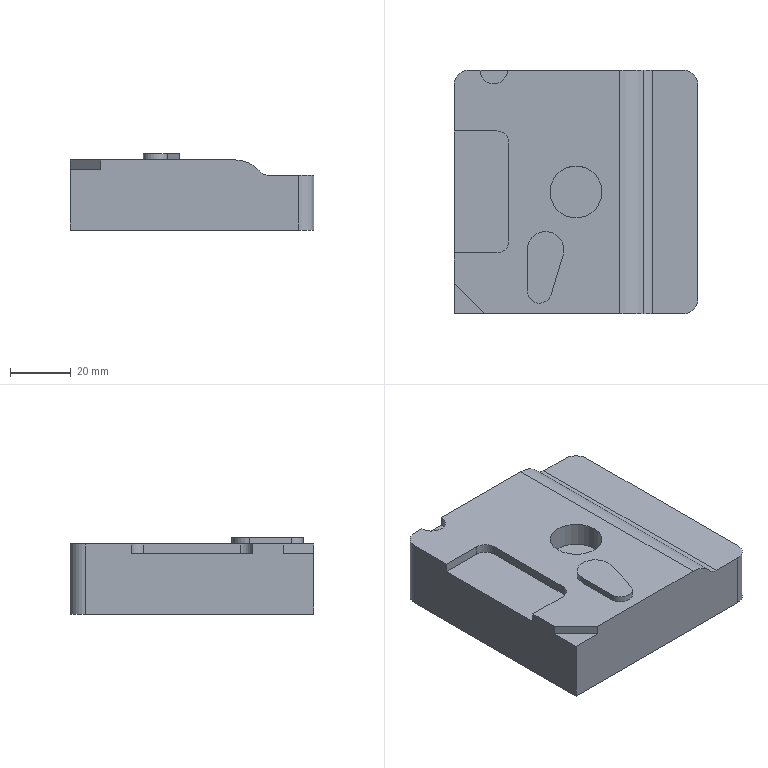NC program | NX | posted with a generic post | part box 80 x 80 x 25 mm
Lines 1 to 1870 of 8300:
N10 G17 G21 G94 G90
(CAVITY_MILL , TOOL : D12D)
N12 T00 M6
N14 G53
N16 G17 G0 G90 X8.231 Y51.991 S0 M3
N18 G43 Z8. H0
N20 Z4.467
N22 G94 G1 Z1.467 F250.
N24 Y41.191
N26 X40.004
N28 G2 X41.191 Y40.004 R1.213
N30 G1 Y-40.004
N32 G2 X40.004 Y-41.191 R1.213
N34 G1 X-4.685
N36 G3 X-1.128 Y-35.794 R11.36
N38 G1 X2.786 Y-22.874
N40 G3 X-23.36 Y-19. R-13.36
N42 G1 Y-32.5
N44 G3 X-19.315 Y-41.191 R11.36
N46 G1 X-18.697 Y-40.457
N48 G2 X-22.4 Y-32.5 R10.4
N50 G1 Y-19.
N52 G2 X1.867 Y-22.595 R-12.4
N54 G1 X-2.047 Y-35.515
N56 G2 X-18.697 Y-40.457 R10.4
N58 G1 X-19.315 Y-41.191
N60 X-40.036
N62 X-40.038
N64 G2 X-40.453 Y-41.11 R1.095
N66 X-41.11 Y-40.453 R1.431
N68 X-41.191 Y-40.038 R1.095
N70 G1 Y-40.036
N72 Y40.004
N74 G2 X-40.004 Y41.191 R1.213
N76 G1 X8.231
N78 Y36.391
N80 X36.391
N82 Y-36.391
N84 X3.706
N86 X7.38 Y-24.265
N88 G3 X-28.16 Y-19. R-18.16
N90 G1 Y-32.5
N92 G3 X-27.684 Y-36.391 R16.16
N94 G1 X-36.391
N96 Y36.391
N98 X8.231
N100 Y31.591
N102 X31.591
N104 Y-31.591
N106 X10.176
N108 X11.974 Y-25.657
N110 G3 X-31.591 Y-11.191 R22.96
N112 G1 Y31.591
N114 X8.231
N116 Y26.791
N118 X26.791
N120 Y-26.791
N122 X16.644
N124 G3 X-26.791 Y3.106 R27.76
N126 G1 Y26.791
N128 X8.231
N130 Y21.991
N132 X21.991
N134 Y-12.942
N136 G3 X-21.991 Y11.271 R32.56
N138 G1 Y21.991
N140 X8.231
N142 Y17.191
N144 X17.191
N146 Y6.62
N148 G3 X-0.729 Y17.191 R37.36
N150 G1 X8.231
N152 Y23.191
N154 Z4.467
N156 G0 Z8.
N158 Y51.992
N160 Z3.933
N162 G1 Z0.933
N164 Y41.192
N166 X40.004
N168 G2 X41.192 Y40.004 R1.213
N170 G1 Y-40.004
N172 G2 X40.004 Y-41.192 R1.213
N174 G1 X-4.685
N176 G3 X-1.128 Y-35.794 R11.36
N178 G1 X2.786 Y-22.874
N180 G3 X-23.36 Y-19. R-13.36
N182 G1 Y-32.5
N184 G3 X-19.315 Y-41.192 R11.36
N186 G1 X-18.697 Y-40.457
N188 G2 X-22.4 Y-32.5 R10.4
N190 G1 Y-19.
N192 G2 X1.867 Y-22.595 R-12.4
N194 G1 X-2.047 Y-35.515
N196 G2 X-18.697 Y-40.457 R10.4
N198 G1 X-19.315 Y-41.192
N200 X-40.036
N202 X-40.037
N204 G2 X-40.453 Y-41.11 R1.097
N206 X-41.11 Y-40.453 R1.43
N208 X-41.192 Y-40.037 R1.097
N210 G1 Y-40.036
N212 Y40.004
N214 G2 X-40.004 Y41.192 R1.213
N216 G1 X8.231
N218 Y36.392
N220 X36.392
N222 Y-36.392
N224 X3.706
N226 X7.38 Y-24.265
N228 G3 X-28.16 Y-19. R-18.16
N230 G1 Y-32.5
N232 G3 X-27.684 Y-36.392 R16.16
N234 G1 X-36.392
N236 Y36.392
N238 X8.231
N240 Y31.592
N242 X31.592
N244 Y-31.592
N246 X10.176
N248 X11.974 Y-25.657
N250 G3 X-31.592 Y-11.192 R22.96
N252 G1 Y31.592
N254 X8.231
N256 Y26.792
N258 X26.792
N260 Y-26.792
N262 X16.644
N264 G3 X-26.792 Y3.106 R27.76
N266 G1 Y26.792
N268 X8.231
N270 Y21.992
N272 X21.992
N274 Y-12.943
N276 G3 X-21.992 Y11.271 R32.56
N278 G1 Y21.992
N280 X8.231
N282 Y17.192
N284 X17.192
N286 Y6.62
N288 G3 X-0.73 Y17.192 R37.36
N290 G1 X8.231
N292 Y23.192
N294 Z3.933
N296 G0 Z8.
N298 Y51.992
N300 Z3.4
N302 G1 Z0.4
N304 Y41.192
N306 X40.004
N308 G2 X41.192 Y40.004 R1.214
N310 G1 Y-40.004
N312 G2 X40.004 Y-41.192 R1.214
N314 G1 X-4.685
N316 G3 X-1.128 Y-35.794 R11.36
N318 G1 X2.786 Y-22.874
N320 G3 X-23.36 Y-19. R-13.36
N322 G1 Y-32.5
N324 G3 X-19.315 Y-41.192 R11.36
N326 G1 X-18.696 Y-40.457
N328 G2 X-22.4 Y-32.5 R10.4
N330 G1 Y-19.
N332 G2 X1.867 Y-22.595 R-12.4
N334 G1 X-2.047 Y-35.515
N336 G2 X-18.696 Y-40.457 R10.4
N338 G1 X-19.315 Y-41.192
N340 X-40.036
N342 X-40.037
N344 G2 X-40.454 Y-41.11 R1.1
N346 X-41.11 Y-40.454 R1.428
N348 X-41.192 Y-40.037 R1.1
N350 G1 Y-40.036
N352 Y40.004
N354 G2 X-40.004 Y41.192 R1.214
N356 G1 X8.231
N358 Y36.392
N360 X36.392
N362 Y-36.392
N364 X3.706
N366 X7.38 Y-24.265
N368 G3 X-28.16 Y-19. R-18.16
N370 G1 Y-32.5
N372 G3 X-27.684 Y-36.392 R16.16
N374 G1 X-36.392
N376 Y36.392
N378 X8.231
N380 Y31.592
N382 X31.592
N384 Y-31.592
N386 X10.176
N388 X11.974 Y-25.657
N390 G3 X-31.592 Y-11.192 R22.96
N392 G1 Y31.592
N394 X8.231
N396 Y26.792
N398 X26.792
N400 Y-26.792
N402 X16.644
N404 G3 X-26.792 Y3.106 R27.76
N406 G1 Y26.792
N408 X8.231
N410 Y21.992
N412 X21.992
N414 Y-12.944
N416 G3 X-21.992 Y11.271 R32.56
N418 G1 Y21.992
N420 X8.231
N422 Y17.192
N424 X17.192
N426 Y6.62
N428 G3 X-0.73 Y17.192 R37.36
N430 G1 X8.231
N432 Y23.192
N434 Z3.4
N436 G0 Z8.
N438 X51.992 Y0.
N440 Z2.8
N442 G1 Z-0.2
N444 X41.192
N446 Y-40.004
N448 G2 X40.004 Y-41.192 R1.214
N450 G1 X23.68
N452 G3 X23.821 Y-39.864 R6.415
N454 G1 Y39.864
N456 G3 X23.68 Y41.192 R6.415
N458 G1 X40.004
N460 G2 X41.192 Y40.004 R1.214
N462 G1 Y0.
N464 X36.392
N466 Y-36.392
N468 X28.621
N470 Y36.392
N472 X36.392
N474 Y0.
N476 X51.992
N478 Z2.8
N480 G0 Z8.
N482 Z2.2
N484 G1 Z-0.8
N486 X41.192
N488 Y-40.003
N490 G2 X40.003 Y-41.192 R1.214
N492 G1 X25.069
N494 G3 X25.19 Y-39.873 R6.258
N496 G1 Y39.873
N498 G3 X25.071 Y41.192 R6.208
N500 G1 X40.003
N502 G2 X41.192 Y40.003 R1.214
N504 G1 Y0.
N506 X36.392
N508 Y-36.392
N510 X29.99
N512 Y36.392
N514 X36.392
N516 Y0.
N518 X51.992
N520 Z2.2
N522 G0 Z8.
N524 Z1.6
N526 G1 Z-1.4
N528 X41.192
N530 Y-40.003
N532 G2 X40.003 Y-41.192 R1.215
N534 G1 X26.043
N536 G3 X26.188 Y-39.731 R6.584
N538 G1 Y39.731
N540 G3 X26.043 Y41.192 R6.584
N542 G1 X40.003
N544 G2 X41.192 Y40.003 R1.215
N546 G1 Y0.
N548 X36.392
N550 Y-36.392
N552 X30.988
N554 Y36.392
N556 X36.392
N558 Y0.
N560 X51.992
N562 Z1.6
N564 G0 Z8.
N566 X51.993 Z1.
N568 G1 Z-2.
N570 X41.193
N572 Y-40.003
N574 G2 X40.003 Y-41.193 R1.215
N576 G1 X26.865
N578 G3 X26.985 Y-39.873 R6.36
N580 G1 Y39.873
N582 G3 X26.865 Y41.193 R6.365
N584 G1 X40.003
N586 G2 X41.193 Y40.003 R1.215
N588 G1 Y0.
N590 X36.393
N592 Y-36.393
N594 X31.785
N596 Y36.393
N598 X36.393
N600 Y0.
N602 X51.993
N604 Z1.
N606 G0 Z8.
N608 Z0.4
N610 G1 Z-2.6
N612 X41.193
N614 Y-40.003
N616 G2 X40.003 Y-41.193 R1.216
N618 G1 X27.517
N620 G3 X27.64 Y-39.874 R6.426
N622 G1 Y39.874
N624 G3 X27.519 Y41.193 R6.397
N626 G1 X40.003
N628 G2 X41.193 Y40.003 R1.216
N630 G1 Y0.
N632 X36.393
N634 Y-36.393
N636 X32.44
N638 Y36.393
N640 X36.393
N642 Y0.
N644 X51.993
N646 Z0.4
N648 G0 Z8.
N650 Z-0.1
N652 G1 Z-3.1
N654 X41.193
N656 Y-40.003
N658 G2 X40.003 Y-41.193 R1.216
N660 G1 X28.009
N662 G3 X28.121 Y-39.873 R6.314
N664 G1 Y39.873
N666 G3 X28.009 Y41.193 R6.314
N668 G1 X40.003
N670 G2 X41.193 Y40.003 R1.216
N672 G1 Y0.
N674 X36.393
N676 Y-36.393
N678 X32.921
N680 Y36.393
N682 X36.393
N684 Y0.
N686 X51.993
N688 Z-0.1
N690 G0 Z8.
N692 Z-0.6
N694 G1 Z-3.6
N696 X41.193
N698 Y-40.003
N700 G2 X40.003 Y-41.193 R1.216
N702 G1 X28.478
N704 G3 X28.574 Y-39.806 R6.174
N706 G1 Y39.806
N708 G3 X28.478 Y41.193 R6.174
N710 G1 X40.003
N712 G2 X41.193 Y40.003 R1.216
N714 G1 Y0.
N716 X36.393
N718 Y-36.393
N720 X33.374
N722 Y36.393
N724 X36.393
N726 Y0.
N728 X51.993
N730 Z-0.6
N732 G0 Z8.
N734 Z-1.1
N736 G1 Z-4.1
N738 X41.193
N740 Y-40.003
N742 G2 X40.003 Y-41.193 R1.217
N744 G1 X29.129
N746 G3 X29.234 Y-39.873 R6.204
N748 G1 Y39.873
N750 G3 X29.129 Y41.193 R6.204
N752 G1 X40.003
N754 G2 X41.193 Y40.003 R1.217
N756 G1 Y0.
N758 X36.393
N760 Y-36.393
N762 X34.034
N764 Y36.393
N766 X36.393
N768 Y0.
N770 X51.993
N772 Z-1.1
N774 G0 Z8.
N776 X51.994 Z-1.6
N778 G1 Z-4.6
N780 X41.194
N782 Y-40.003
N784 G2 X40.003 Y-41.194 R1.217
N786 G1 X30.774
N788 G3 X30.832 Y-39.876 R5.623
N790 G1 Y39.876
N792 G3 X30.781 Y41.194 R5.507
N794 G1 X40.003
N796 G2 X41.194 Y40.003 R1.217
N798 G1 Y0.
N800 X36.394
N802 Y-36.394
N804 X35.632
N806 Y36.394
N808 X36.394
N810 Y0.
N812 X51.994
N814 Z-1.6
N816 G0 Z8.
N818 X32.23 Y52.4
N820 Z-2.2
N822 G1 Z-5.2
N824 Y47.581
N826 X38.016 Y45.994
N828 G2 X45.994 Y38.016 R11.4
N830 G1 X47.581 Y32.23
N832 X52.4
N834 Z-2.2
N836 G0 Z8.
N838 X32.229 Y52.4
N840 Z-2.8
N842 G1 Z-5.8
N844 Y47.581
N846 X38.016 Y45.994
N848 G2 X45.994 Y38.016 R11.4
N850 G1 X47.581 Y32.229
N852 X52.4
N854 Z-2.8
N856 G0 Z8.
N858 X32.228 Y52.4
N860 Z-3.4
N862 G1 Z-6.4
N864 Y47.581
N866 X38.015 Y45.994
N868 G2 X45.994 Y38.015 R11.4
N870 G1 X47.581 Y32.228
N872 X52.4
N874 Z-3.4
N876 G0 Z8.
N878 X32.228 Y52.4
N880 Z-4.
N882 G1 Z-7.
N884 Y47.581
N886 X38.014 Y45.994
N888 G2 X45.994 Y38.014 R11.4
N890 G1 X47.581 Y32.228
N892 X52.4
N894 Z-4.
N896 G0 Z8.
N898 X32.227 Y52.4
N900 Z-4.6
N902 G1 Z-7.6
N904 Y47.58
N906 X38.013 Y45.995
N908 G2 X45.995 Y38.013 R11.4
N910 G1 X47.58 Y32.227
N912 X52.4
N914 Z-4.6
N916 G0 Z8.
N918 X32.226 Y52.4
N920 Z-5.192
N922 G1 Z-8.192
N924 Y47.58
N926 X38.013 Y45.995
N928 G2 X45.995 Y38.013 R11.4
N930 G1 X47.58 Y32.226
N932 X52.4
N934 Z-5.192
N936 G0 Z8.
N938 X32.225 Y52.4
N940 Z-5.785
N942 G1 Z-8.785
N944 Y47.58
N946 X38.012 Y45.995
N948 G2 X45.995 Y38.012 R11.4
N950 G1 X47.58 Y32.225
N952 X52.4
N954 Z-5.785
N956 G0 Z8.
N958 X32.224 Y52.4
N960 Z-6.377
N962 G1 Z-9.377
N964 Y47.58
N966 X38.011 Y45.995
N968 G2 X45.995 Y38.011 R11.4
N970 G1 X47.58 Y32.224
N972 X52.4
N974 Z-6.377
N976 G0 Z8.
N978 X32.223 Y52.4
N980 Z-6.969
N982 G1 Z-9.969
N984 Y47.58
N986 X38.01 Y45.995
N988 G2 X45.995 Y38.01 R11.4
N990 G1 X47.58 Y32.223
N992 X52.4
N994 Z-6.969
N996 G0 Z8.
N998 X32.222 Y52.4
N1000 Z-7.562
N1002 G1 Z-10.562
N1004 Y47.58
N1006 X38.01 Y45.996
N1008 G2 X45.996 Y38.01 R11.4
N1010 G1 X47.58 Y32.222
N1012 X52.4
N1014 Z-7.562
N1016 G0 Z8.
N1018 X32.222 Y52.4
N1020 Z-8.154
N1022 G1 Z-11.154
N1024 Y47.579
N1026 X38.009 Y45.996
N1028 G2 X45.996 Y38.009 R11.4
N1030 G1 X47.579 Y32.222
N1032 X52.4
N1034 Z-8.154
N1036 G0 Z8.
N1038 X32.221 Y52.4
N1040 Z-8.746
N1042 G1 Z-11.746
N1044 Y47.579
N1046 X38.008 Y45.996
N1048 G2 X45.996 Y38.008 R11.4
N1050 G1 X47.579 Y32.221
N1052 X52.4
N1054 Z-8.746
N1056 G0 Z8.
N1058 X32.22 Y52.4
N1060 Z-9.338
N1062 G1 Z-12.338
N1064 Y47.579
N1066 X38.007 Y45.996
N1068 G2 X45.996 Y38.007 R11.4
N1070 G1 X47.579 Y32.22
N1072 X52.4
N1074 Z-9.338
N1076 G0 Z8.
N1078 X32.219 Y52.4
N1080 Z-9.931
N1082 G1 Z-12.931
N1084 Y47.579
N1086 X38.007 Y45.996
N1088 G2 X45.996 Y38.007 R11.4
N1090 G1 X47.579 Y32.219
N1092 X52.4
N1094 Z-9.931
N1096 G0 Z8.
N1098 X32.218 Y52.4
N1100 Z-10.523
N1102 G1 Z-13.523
N1104 Y47.579
N1106 X38.006 Y45.997
N1108 G2 X45.997 Y38.006 R11.4
N1110 G1 X47.579 Y32.218
N1112 X52.4
N1114 Z-10.523
N1116 G0 Z8.
N1118 X32.217 Y52.4
N1120 Z-11.115
N1122 G1 Z-14.115
N1124 Y47.578
N1126 X38.005 Y45.997
N1128 G2 X45.997 Y38.005 R11.4
N1130 G1 X47.578 Y32.217
N1132 X52.4
N1134 Z-11.115
N1136 G0 Z8.
N1138 X32.216 Y52.4
N1140 Z-11.708
N1142 G1 Z-14.708
N1144 Y47.578
N1146 X38.004 Y45.997
N1148 G2 X45.997 Y38.004 R11.4
N1150 G1 X47.578 Y32.216
N1152 X52.4
N1154 Z-11.708
N1156 G0 Z8.
N1158 X32.216 Y52.4
N1160 Z-12.3
N1162 G1 Z-15.3
N1164 Y47.578
N1166 X38.004 Y45.997
N1168 G2 X45.997 Y38.004 R11.4
N1170 G1 X47.578 Y32.216
N1172 X52.4
N1174 Z-12.3
N1176 G0 Z8.
N1178 X32.215 Y52.4
N1180 Z-12.892
N1182 G1 Z-15.892
N1184 Y47.578
N1186 X38.003 Y45.997
N1188 G2 X45.997 Y38.003 R11.4
N1190 G1 X47.578 Y32.215
N1192 X52.4
N1194 Z-12.892
N1196 G0 Z8.
N1198 X32.214 Y52.4
N1200 Z-13.485
N1202 G1 Z-16.485
N1204 Y47.578
N1206 X38.002 Y45.998
N1208 G2 X45.998 Y38.002 R11.4
N1210 G1 X47.578 Y32.214
N1212 X52.4
N1214 Z-13.485
N1216 G0 Z8.
N1218 X32.213 Y52.4
N1220 Z-14.077
N1222 G1 Z-17.077
N1224 Y47.577
N1226 X38.001 Y45.998
N1228 G2 X45.998 Y38.001 R11.4
N1230 G1 X47.577 Y32.213
N1232 X52.4
N1234 Z-14.077
N1236 G0 Z8.
N1238 X32.212 Y52.4
N1240 Z-14.669
N1242 G1 Z-17.669
N1244 Y47.577
N1246 X38.001 Y45.998
N1248 G2 X45.998 Y38.001 R11.4
N1250 G1 X47.577 Y32.212
N1252 X52.4
N1254 Z-14.669
N1256 G0 Z8.
N1258 X32.211 Y52.4
N1260 Z-15.262
N1262 G1 Z-18.262
N1264 Y47.577
N1266 X38. Y45.998
N1268 G2 X45.998 Y38. R11.4
N1270 G1 X47.577 Y32.211
N1272 X52.4
N1274 Z-15.262
N1276 G0 Z8.
N1278 X32.21 Y52.4
N1280 Z-15.854
N1282 G1 Z-18.854
N1284 Y47.577
N1286 X37.999 Y45.998
N1288 G2 X45.998 Y37.999 R11.4
N1290 G1 X47.577 Y32.21
N1292 X52.4
N1294 Z-15.854
N1296 G0 Z8.
N1298 X32.209 Y52.4
N1300 Z-16.446
N1302 G1 Z-19.446
N1304 Y47.577
N1306 X37.998 Y45.999
N1308 G2 X45.999 Y37.998 R11.4
N1310 G1 X47.577 Y32.209
N1312 X52.4
N1314 Z-16.446
N1316 G0 Z8.
N1318 X32.209 Y52.4
N1320 Z-17.038
N1322 G1 Z-20.038
N1324 Y47.576
N1326 X37.997 Y45.999
N1328 G2 X45.999 Y37.997 R11.4
N1330 G1 X47.576 Y32.209
N1332 X52.4
N1334 Z-17.038
N1336 G0 Z8.
N1338 X32.208 Y52.4
N1340 Z-17.631
N1342 G1 Z-20.631
N1344 Y47.576
N1346 X37.997 Y45.999
N1348 G2 X45.999 Y37.997 R11.4
N1350 G1 X47.576 Y32.208
N1352 X52.4
N1354 Z-17.631
N1356 G0 Z8.
N1358 X32.207 Y52.4
N1360 Z-18.223
N1362 G1 Z-21.223
N1364 Y47.576
N1366 X37.996 Y45.999
N1368 G2 X45.999 Y37.996 R11.4
N1370 G1 X47.576 Y32.207
N1372 X52.4
N1374 Z-18.223
N1376 G0 Z8.
N1378 X32.206 Y52.4
N1380 Z-18.815
N1382 G1 Z-21.815
N1384 Y47.576
N1386 X37.995 Y45.999
N1388 G2 X45.999 Y37.995 R11.4
N1390 G1 X47.576 Y32.206
N1392 X52.4
N1394 Z-18.815
N1396 G0 Z8.
N1398 X32.205 Y52.4
N1400 Z-19.408
N1402 G1 Z-22.408
N1404 Y47.576
N1406 X37.994 Y46.
N1408 G2 X46. Y37.994 R11.4
N1410 G1 X47.576 Y32.205
N1412 X52.4
N1414 Z-19.408
N1416 G0 Z8.
N1418 X32.204 Y52.4
N1420 Z-20.
N1422 G1 Z-23.
N1424 Y47.576
N1426 X37.994 Y46.
N1428 G2 X46. Y37.994 R11.4
N1430 G1 X47.576 Y32.204
N1432 X52.4
N1434 Z-20.
N1436 G0 Z8.
N1438 Y-32.23
N1440 Z-2.2
N1442 G1 Z-5.2
N1444 X47.581
N1446 X45.994 Y-38.016
N1448 G2 X38.016 Y-45.994 R11.4
N1450 G1 X32.23 Y-47.581
N1452 Y-52.4
N1454 Z-2.2
N1456 G0 Z8.
N1458 X52.4 Y-32.229
N1460 Z-2.8
N1462 G1 Z-5.8
N1464 X47.581
N1466 X45.994 Y-38.016
N1468 G2 X38.016 Y-45.994 R11.4
N1470 G1 X32.229 Y-47.581
N1472 Y-52.4
N1474 Z-2.8
N1476 G0 Z8.
N1478 X52.4 Y-32.228
N1480 Z-3.4
N1482 G1 Z-6.4
N1484 X47.581
N1486 X45.994 Y-38.015
N1488 G2 X38.015 Y-45.994 R11.4
N1490 G1 X32.228 Y-47.581
N1492 Y-52.4
N1494 Z-3.4
N1496 G0 Z8.
N1498 X52.4 Y-32.228
N1500 Z-4.
N1502 G1 Z-7.
N1504 X47.581
N1506 X45.994 Y-38.014
N1508 G2 X38.014 Y-45.994 R11.4
N1510 G1 X32.228 Y-47.581
N1512 Y-52.4
N1514 Z-4.
N1516 G0 Z8.
N1518 X52.4 Y-32.227
N1520 Z-4.6
N1522 G1 Z-7.6
N1524 X47.58
N1526 X45.995 Y-38.013
N1528 G2 X38.013 Y-45.995 R11.4
N1530 G1 X32.227 Y-47.58
N1532 Y-52.4
N1534 Z-4.6
N1536 G0 Z8.
N1538 X52.4 Y-32.226
N1540 Z-5.192
N1542 G1 Z-8.192
N1544 X47.58
N1546 X45.995 Y-38.013
N1548 G2 X38.013 Y-45.995 R11.4
N1550 G1 X32.226 Y-47.58
N1552 Y-52.4
N1554 Z-5.192
N1556 G0 Z8.
N1558 X52.4 Y-32.225
N1560 Z-5.785
N1562 G1 Z-8.785
N1564 X47.58
N1566 X45.995 Y-38.012
N1568 G2 X38.012 Y-45.995 R11.4
N1570 G1 X32.225 Y-47.58
N1572 Y-52.4
N1574 Z-5.785
N1576 G0 Z8.
N1578 X52.4 Y-32.224
N1580 Z-6.377
N1582 G1 Z-9.377
N1584 X47.58
N1586 X45.995 Y-38.011
N1588 G2 X38.011 Y-45.995 R11.4
N1590 G1 X32.224 Y-47.58
N1592 Y-52.4
N1594 Z-6.377
N1596 G0 Z8.
N1598 X52.4 Y-32.223
N1600 Z-6.969
N1602 G1 Z-9.969
N1604 X47.58
N1606 X45.995 Y-38.01
N1608 G2 X38.01 Y-45.995 R11.4
N1610 G1 X32.223 Y-47.58
N1612 Y-52.4
N1614 Z-6.969
N1616 G0 Z8.
N1618 X52.4 Y-32.222
N1620 Z-7.562
N1622 G1 Z-10.562
N1624 X47.58
N1626 X45.996 Y-38.01
N1628 G2 X38.01 Y-45.996 R11.4
N1630 G1 X32.222 Y-47.58
N1632 Y-52.4
N1634 Z-7.562
N1636 G0 Z8.
N1638 X52.4 Y-32.222
N1640 Z-8.154
N1642 G1 Z-11.154
N1644 X47.579
N1646 X45.996 Y-38.009
N1648 G2 X38.009 Y-45.996 R11.4
N1650 G1 X32.222 Y-47.579
N1652 Y-52.4
N1654 Z-8.154
N1656 G0 Z8.
N1658 X52.4 Y-32.221
N1660 Z-8.746
N1662 G1 Z-11.746
N1664 X47.579
N1666 X45.996 Y-38.008
N1668 G2 X38.008 Y-45.996 R11.4
N1670 G1 X32.221 Y-47.579
N1672 Y-52.4
N1674 Z-8.746
N1676 G0 Z8.
N1678 X52.4 Y-32.22
N1680 Z-9.338
N1682 G1 Z-12.338
N1684 X47.579
N1686 X45.996 Y-38.007
N1688 G2 X38.007 Y-45.996 R11.4
N1690 G1 X32.22 Y-47.579
N1692 Y-52.4
N1694 Z-9.338
N1696 G0 Z8.
N1698 X52.4 Y-32.219
N1700 Z-9.931
N1702 G1 Z-12.931
N1704 X47.579
N1706 X45.996 Y-38.007
N1708 G2 X38.007 Y-45.996 R11.4
N1710 G1 X32.219 Y-47.579
N1712 Y-52.4
N1714 Z-9.931
N1716 G0 Z8.
N1718 X52.4 Y-32.218
N1720 Z-10.523
N1722 G1 Z-13.523
N1724 X47.579
N1726 X45.997 Y-38.006
N1728 G2 X38.006 Y-45.997 R11.4
N1730 G1 X32.218 Y-47.579
N1732 Y-52.4
N1734 Z-10.523
N1736 G0 Z8.
N1738 X52.4 Y-32.217
N1740 Z-11.115
N1742 G1 Z-14.115
N1744 X47.578
N1746 X45.997 Y-38.005
N1748 G2 X38.005 Y-45.997 R11.4
N1750 G1 X32.217 Y-47.578
N1752 Y-52.4
N1754 Z-11.115
N1756 G0 Z8.
N1758 X52.4 Y-32.216
N1760 Z-11.708
N1762 G1 Z-14.708
N1764 X47.578
N1766 X45.997 Y-38.004
N1768 G2 X38.004 Y-45.997 R11.4
N1770 G1 X32.216 Y-47.578
N1772 Y-52.4
N1774 Z-11.708
N1776 G0 Z8.
N1778 X52.4 Y-32.216
N1780 Z-12.3
N1782 G1 Z-15.3
N1784 X47.578
N1786 X45.997 Y-38.004
N1788 G2 X38.004 Y-45.997 R11.4
N1790 G1 X32.216 Y-47.578
N1792 Y-52.4
N1794 Z-12.3
N1796 G0 Z8.
N1798 X52.4 Y-32.215
N1800 Z-12.892
N1802 G1 Z-15.892
N1804 X47.578
N1806 X45.997 Y-38.003
N1808 G2 X38.003 Y-45.997 R11.4
N1810 G1 X32.215 Y-47.578
N1812 Y-52.4
N1814 Z-12.892
N1816 G0 Z8.
N1818 X52.4 Y-32.214
N1820 Z-13.485
N1822 G1 Z-16.485
N1824 X47.578
N1826 X45.998 Y-38.002
N1828 G2 X38.002 Y-45.998 R11.4
N1830 G1 X32.214 Y-47.578
N1832 Y-52.4
N1834 Z-13.485
N1836 G0 Z8.
N1838 X52.4 Y-32.213
N1840 Z-14.077
N1842 G1 Z-17.077
N1844 X47.577
N1846 X45.998 Y-38.001
N1848 G2 X38.001 Y-45.998 R11.4
N1850 G1 X32.213 Y-47.577
N1852 Y-52.4
N1854 Z-14.077
N1856 G0 Z8.
N1858 X52.4 Y-32.212
N1860 Z-14.669
N1862 G1 Z-17.669
N1864 X47.577
N1866 X45.998 Y-38.001
N1868 G2 X38.001 Y-45.998 R11.4
N1870 G1 X32.212 Y-47.577
N1872 Y-52.4
N1874 Z-14.669
N1876 G0 Z8.
N1878 X52.4 Y-32.211
N1880 Z-15.262
N1882 G1 Z-18.262
N1884 X47.577
N1886 X45.998 Y-38.
N1888 G2 X38. Y-45.998 R11.4
N1890 G1 X32.211 Y-47.577
N1892 Y-52.4
N1894 Z-15.262
N1896 G0 Z8.
N1898 X52.4 Y-32.21
N1900 Z-15.854
N1902 G1 Z-18.854
N1904 X47.577
N1906 X45.998 Y-37.999
N1908 G2 X37.999 Y-45.998 R11.4
N1910 G1 X32.21 Y-47.577
N1912 Y-52.4
N1914 Z-15.854
N1916 G0 Z8.
N1918 X52.4 Y-32.209
N1920 Z-16.446
N1922 G1 Z-19.446
N1924 X47.577
N1926 X45.999 Y-37.998
N1928 G2 X37.998 Y-45.999 R11.4
N1930 G1 X32.209 Y-47.577
N1932 Y-52.4
N1934 Z-16.446
N1936 G0 Z8.
N1938 X52.4 Y-32.209
N1940 Z-17.038
N1942 G1 Z-20.038
N1944 X47.576
N1946 X45.999 Y-37.997
N1948 G2 X37.997 Y-45.999 R11.4
N1950 G1 X32.209 Y-47.576
N1952 Y-52.4
N1954 Z-17.038
N1956 G0 Z8.
N1958 X52.4 Y-32.208
N1960 Z-17.631
N1962 G1 Z-20.631
N1964 X47.576
N1966 X45.999 Y-37.997
N1968 G2 X37.997 Y-45.999 R11.4
N1970 G1 X32.208 Y-47.576
N1972 Y-52.4
N1974 Z-17.631
N1976 G0 Z8.
N1978 X52.4 Y-32.207
N1980 Z-18.223
N1982 G1 Z-21.223
N1984 X47.576
N1986 X45.999 Y-37.996
N1988 G2 X37.996 Y-45.999 R11.4
N1990 G1 X32.207 Y-47.576
N1992 Y-52.4
N1994 Z-18.223
N1996 G0 Z8.
N1998 X52.4 Y-32.206
N2000 Z-18.815
N2002 G1 Z-21.815
N2004 X47.576
N2006 X45.999 Y-37.995
N2008 G2 X37.995 Y-45.999 R11.4
N2010 G1 X32.206 Y-47.576
N2012 Y-52.4
N2014 Z-18.815
N2016 G0 Z8.
N2018 X52.4 Y-32.205
N2020 Z-19.408
N2022 G1 Z-22.408
N2024 X47.576
N2026 X46. Y-37.994
N2028 G2 X37.994 Y-46. R11.4
N2030 G1 X32.205 Y-47.576
N2032 Y-52.4
N2034 Z-19.408
N2036 G0 Z8.
N2038 X52.4 Y-32.204
N2040 Z-20.
N2042 G1 Z-23.
N2044 X47.576
N2046 X46. Y-37.994
N2048 G2 X37.994 Y-46. R11.4
N2050 G1 X32.204 Y-47.576
N2052 Y-52.4
N2054 Z-20.
N2056 G0 Z8.
N2058 X-1.835 Y1.021
N2060 Z3.4
N2062 G2 X-1.835 Y1.021 Z3.054 I1.835 J-1.021
N2064 X-1.835 Y1.021 Z2.709 I1.835 J-1.021
N2066 X-1.835 Y1.021 Z2.363 I1.835 J-1.021
N2068 X-1.835 Y1.021 Z2.018 I1.835 J-1.021
N2070 X-1.835 Y1.021 Z1.672 I1.835 J-1.021
N2072 X-1.835 Y1.021 Z1.327 I1.835 J-1.021
N2074 X-1.835 Y1.021 Z0.981 I1.835 J-1.021
N2076 X-1.835 Y1.021 Z0.636 I1.835 J-1.021
N2078 X-1.835 Y1.021 Z0.29 I1.835 J-1.021
N2080 X-1.835 Y1.021 Z-0.055 I1.835 J-1.021
N2082 X2.1 Y0. Z-0.2 R2.1
N2084 X0. Y-2.1 R2.1
N2086 X2.1 Y0. R-2.1
N2088 G1 Z2.8
N2090 G0 Z8.
N2092 X-1.835 Y1.021
N2094 Z2.8
N2096 G2 X-1.835 Y1.021 Z2.454 I1.835 J-1.021
N2098 X-1.835 Y1.021 Z2.109 I1.835 J-1.021
N2100 X-1.835 Y1.021 Z1.763 I1.835 J-1.021
N2102 X-1.835 Y1.021 Z1.418 I1.835 J-1.021
N2104 X-1.835 Y1.021 Z1.072 I1.835 J-1.021
N2106 X-1.835 Y1.021 Z0.727 I1.835 J-1.021
N2108 X-1.835 Y1.021 Z0.381 I1.835 J-1.021
N2110 X-1.835 Y1.021 Z0.036 I1.835 J-1.021
N2112 X-1.835 Y1.021 Z-0.31 I1.835 J-1.021
N2114 X-1.835 Y1.021 Z-0.655 I1.835 J-1.021
N2116 X2.1 Y0. Z-0.8 R2.1
N2118 X0. Y-2.1 R2.1
N2120 X2.1 Y0. R-2.1
N2122 G1 Z2.2
N2124 G0 Z8.
N2126 X-1.835 Y1.021
N2128 Z2.2
N2130 G2 X-1.835 Y1.021 Z1.854 I1.835 J-1.021
N2132 X-1.835 Y1.021 Z1.509 I1.835 J-1.021
N2134 X-1.835 Y1.021 Z1.163 I1.835 J-1.021
N2136 X-1.835 Y1.021 Z0.818 I1.835 J-1.021
N2138 X-1.835 Y1.021 Z0.472 I1.835 J-1.021
N2140 X-1.835 Y1.021 Z0.127 I1.835 J-1.021
N2142 X-1.835 Y1.021 Z-0.219 I1.835 J-1.021
N2144 X-1.835 Y1.021 Z-0.564 I1.835 J-1.021
N2146 X-1.835 Y1.021 Z-0.91 I1.835 J-1.021
N2148 X-1.835 Y1.021 Z-1.255 I1.835 J-1.021
N2150 X2.1 Y0. Z-1.4 R2.1
N2152 X0. Y-2.1 R2.1
N2154 X2.1 Y0. R-2.1
N2156 G1 Z1.6
N2158 G0 Z8.
N2160 X-1.835 Y1.021
N2162 Z1.6
N2164 G2 X-1.835 Y1.021 Z1.254 I1.835 J-1.021
N2166 X-1.835 Y1.021 Z0.909 I1.835 J-1.021
N2168 X-1.835 Y1.021 Z0.563 I1.835 J-1.021
N2170 X-1.835 Y1.021 Z0.218 I1.835 J-1.021
N2172 X-1.835 Y1.021 Z-0.128 I1.835 J-1.021
N2174 X-1.835 Y1.021 Z-0.473 I1.835 J-1.021
N2176 X-1.835 Y1.021 Z-0.819 I1.835 J-1.021
N2178 X-1.835 Y1.021 Z-1.164 I1.835 J-1.021
N2180 X-1.835 Y1.021 Z-1.51 I1.835 J-1.021
N2182 X-1.835 Y1.021 Z-1.855 I1.835 J-1.021
N2184 X2.1 Y0. Z-2. R2.1
N2186 X0. Y-2.1 R2.1
N2188 X2.1 Y0. R-2.1
N2190 G1 Z1.
N2192 G0 Z8.
N2194 X-1.835 Y1.021
N2196 Z1.
N2198 G2 X-1.835 Y1.021 Z0.654 I1.835 J-1.021
N2200 X-1.835 Y1.021 Z0.309 I1.835 J-1.021
N2202 X-1.835 Y1.021 Z-0.037 I1.835 J-1.021
N2204 X-1.835 Y1.021 Z-0.382 I1.835 J-1.021
N2206 X-1.835 Y1.021 Z-0.728 I1.835 J-1.021
N2208 X-1.835 Y1.021 Z-1.073 I1.835 J-1.021
N2210 X-1.835 Y1.021 Z-1.419 I1.835 J-1.021
N2212 X-1.835 Y1.021 Z-1.764 I1.835 J-1.021
N2214 X-1.835 Y1.021 Z-2.11 I1.835 J-1.021
N2216 X-1.835 Y1.021 Z-2.455 I1.835 J-1.021
N2218 X2.1 Y0. Z-2.6 R2.1
N2220 X0. Y-2.1 R2.1
N2222 X2.1 Y0. R-2.1
N2224 G1 Z0.4
N2226 G0 Z8.
N2228 X1.439 Y1.529
N2230 Z0.4
N2232 G2 X1.439 Y1.529 Z0.054 I-1.439 J-1.529
N2234 X1.439 Y1.529 Z-0.291 I-1.439 J-1.529
N2236 X1.439 Y1.529 Z-0.637 I-1.439 J-1.529
N2238 X1.439 Y1.529 Z-0.982 I-1.439 J-1.529
N2240 X1.439 Y1.529 Z-1.328 I-1.439 J-1.529
N2242 X1.439 Y1.529 Z-1.673 I-1.439 J-1.529
N2244 X1.439 Y1.529 Z-2.019 I-1.439 J-1.529
N2246 X1.439 Y1.529 Z-2.364 I-1.439 J-1.529
N2248 X1.439 Y1.529 Z-2.71 I-1.439 J-1.529
N2250 X1.439 Y1.529 Z-3.055 I-1.439 J-1.529
N2252 X2.1 Y0. Z-3.1 R2.1
N2254 X0. Y-2.1 R2.1
N2256 X2.1 Y0. R-2.1
N2258 G1 Z-0.1
N2260 G0 Z8.
N2262 X1.439 Y1.529
N2264 Z-0.1
N2266 G2 X1.439 Y1.529 Z-0.446 I-1.439 J-1.529
N2268 X1.439 Y1.529 Z-0.791 I-1.439 J-1.529
N2270 X1.439 Y1.529 Z-1.137 I-1.439 J-1.529
N2272 X1.439 Y1.529 Z-1.482 I-1.439 J-1.529
N2274 X1.439 Y1.529 Z-1.828 I-1.439 J-1.529
N2276 X1.439 Y1.529 Z-2.173 I-1.439 J-1.529
N2278 X1.439 Y1.529 Z-2.519 I-1.439 J-1.529
N2280 X1.439 Y1.529 Z-2.864 I-1.439 J-1.529
N2282 X1.439 Y1.529 Z-3.21 I-1.439 J-1.529
N2284 X1.439 Y1.529 Z-3.555 I-1.439 J-1.529
N2286 X2.1 Y0. Z-3.6 R2.1
N2288 X0. Y-2.1 R2.1
N2290 X2.1 Y0. R-2.1
N2292 G1 Z-0.6
N2294 G0 Z8.
N2296 X1.439 Y1.529
N2298 Z-0.6
N2300 G2 X1.439 Y1.529 Z-0.946 I-1.439 J-1.529
N2302 X1.439 Y1.529 Z-1.291 I-1.439 J-1.529
N2304 X1.439 Y1.529 Z-1.637 I-1.439 J-1.529
N2306 X1.439 Y1.529 Z-1.982 I-1.439 J-1.529
N2308 X1.439 Y1.529 Z-2.328 I-1.439 J-1.529
N2310 X1.439 Y1.529 Z-2.673 I-1.439 J-1.529
N2312 X1.439 Y1.529 Z-3.019 I-1.439 J-1.529
N2314 X1.439 Y1.529 Z-3.364 I-1.439 J-1.529
N2316 X1.439 Y1.529 Z-3.71 I-1.439 J-1.529
N2318 X1.439 Y1.529 Z-4.055 I-1.439 J-1.529
N2320 X2.1 Y0. Z-4.1 R2.1
N2322 X0. Y-2.1 R2.1
N2324 X2.1 Y0. R-2.1
N2326 G1 Z-1.1
N2328 G0 Z8.
N2330 X1.439 Y1.529
N2332 Z-1.1
N2334 G2 X1.439 Y1.529 Z-1.446 I-1.439 J-1.529
N2336 X1.439 Y1.529 Z-1.791 I-1.439 J-1.529
N2338 X1.439 Y1.529 Z-2.137 I-1.439 J-1.529
N2340 X1.439 Y1.529 Z-2.482 I-1.439 J-1.529
N2342 X1.439 Y1.529 Z-2.828 I-1.439 J-1.529
N2344 X1.439 Y1.529 Z-3.173 I-1.439 J-1.529
N2346 X1.439 Y1.529 Z-3.519 I-1.439 J-1.529
N2348 X1.439 Y1.529 Z-3.864 I-1.439 J-1.529
N2350 X1.439 Y1.529 Z-4.21 I-1.439 J-1.529
N2352 X1.439 Y1.529 Z-4.555 I-1.439 J-1.529
N2354 X2.1 Y0. Z-4.6 R2.1
N2356 X0. Y-2.1 R2.1
N2358 X2.1 Y0. R-2.1
N2360 G1 Z-1.6
N2362 G0 Z8.
N2364 X-1.835 Y1.021
N2366 Z-1.6
N2368 G2 X-1.835 Y1.021 Z-1.946 I1.835 J-1.021
N2370 X-1.835 Y1.021 Z-2.291 I1.835 J-1.021
N2372 X-1.835 Y1.021 Z-2.637 I1.835 J-1.021
N2374 X-1.835 Y1.021 Z-2.982 I1.835 J-1.021
N2376 X-1.835 Y1.021 Z-3.328 I1.835 J-1.021
N2378 X-1.835 Y1.021 Z-3.673 I1.835 J-1.021
N2380 X-1.835 Y1.021 Z-4.019 I1.835 J-1.021
N2382 X-1.835 Y1.021 Z-4.364 I1.835 J-1.021
N2384 X-1.835 Y1.021 Z-4.71 I1.835 J-1.021
N2386 X-1.835 Y1.021 Z-5.055 I1.835 J-1.021
N2388 X2.1 Y0. Z-5.2 R2.1
N2390 X0. Y-2.1 R2.1
N2392 X2.1 Y0. R-2.1
N2394 G1 Z-2.2
N2396 G0 Z8.
N2398 X-1.835 Y1.021
N2400 Z-2.2
N2402 G2 X-1.835 Y1.021 Z-2.546 I1.835 J-1.021
N2404 X-1.835 Y1.021 Z-2.891 I1.835 J-1.021
N2406 X-1.835 Y1.021 Z-3.237 I1.835 J-1.021
N2408 X-1.835 Y1.021 Z-3.582 I1.835 J-1.021
N2410 X-1.835 Y1.021 Z-3.928 I1.835 J-1.021
N2412 X-1.835 Y1.021 Z-4.273 I1.835 J-1.021
N2414 X-1.835 Y1.021 Z-4.619 I1.835 J-1.021
N2416 X-1.835 Y1.021 Z-4.964 I1.835 J-1.021
N2418 X-1.835 Y1.021 Z-5.31 I1.835 J-1.021
N2420 X-1.835 Y1.021 Z-5.655 I1.835 J-1.021
N2422 X2.1 Y0. Z-5.8 R2.1
N2424 X0. Y-2.1 R2.1
N2426 X2.1 Y0. R-2.1
N2428 G1 Z-2.8
N2430 G0 Z8.
N2432 X-1.835 Y1.021
N2434 Z-2.8
N2436 G2 X-1.835 Y1.021 Z-3.146 I1.835 J-1.021
N2438 X-1.835 Y1.021 Z-3.491 I1.835 J-1.021
N2440 X-1.835 Y1.021 Z-3.837 I1.835 J-1.021
N2442 X-1.835 Y1.021 Z-4.182 I1.835 J-1.021
N2444 X-1.835 Y1.021 Z-4.528 I1.835 J-1.021
N2446 X-1.835 Y1.021 Z-4.873 I1.835 J-1.021
N2448 X-1.835 Y1.021 Z-5.219 I1.835 J-1.021
N2450 X-1.835 Y1.021 Z-5.564 I1.835 J-1.021
N2452 X-1.835 Y1.021 Z-5.91 I1.835 J-1.021
N2454 X-1.835 Y1.021 Z-6.255 I1.835 J-1.021
N2456 X2.1 Y0. Z-6.4 R2.1
N2458 X0. Y-2.1 R2.1
N2460 X2.1 Y0. R-2.1
N2462 G1 Z-3.4
N2464 G0 Z8.
N2466 X-1.835 Y1.021
N2468 Z-3.4
N2470 G2 X-1.835 Y1.021 Z-3.746 I1.835 J-1.021
N2472 X-1.835 Y1.021 Z-4.091 I1.835 J-1.021
N2474 X-1.835 Y1.021 Z-4.437 I1.835 J-1.021
N2476 X-1.835 Y1.021 Z-4.782 I1.835 J-1.021
N2478 X-1.835 Y1.021 Z-5.128 I1.835 J-1.021
N2480 X-1.835 Y1.021 Z-5.473 I1.835 J-1.021
N2482 X-1.835 Y1.021 Z-5.819 I1.835 J-1.021
N2484 X-1.835 Y1.021 Z-6.164 I1.835 J-1.021
N2486 X-1.835 Y1.021 Z-6.51 I1.835 J-1.021
N2488 X-1.835 Y1.021 Z-6.855 I1.835 J-1.021
N2490 X2.1 Y0. Z-7. R2.1
N2492 X0. Y-2.1 R2.1
N2494 X2.1 Y0. R-2.1
N2496 G1 Z-4.
N2498 G0 Z8.
N2500 X-1.835 Y1.021
N2502 Z-4.
N2504 G2 X-1.835 Y1.021 Z-4.346 I1.835 J-1.021
N2506 X-1.835 Y1.021 Z-4.691 I1.835 J-1.021
N2508 X-1.835 Y1.021 Z-5.037 I1.835 J-1.021
N2510 X-1.835 Y1.021 Z-5.382 I1.835 J-1.021
N2512 X-1.835 Y1.021 Z-5.728 I1.835 J-1.021
N2514 X-1.835 Y1.021 Z-6.073 I1.835 J-1.021
N2516 X-1.835 Y1.021 Z-6.419 I1.835 J-1.021
N2518 X-1.835 Y1.021 Z-6.764 I1.835 J-1.021
N2520 X-1.835 Y1.021 Z-7.11 I1.835 J-1.021
N2522 X-1.835 Y1.021 Z-7.455 I1.835 J-1.021
N2524 X2.1 Y0. Z-7.6 R2.1
N2526 X0. Y-2.1 R2.1
N2528 X2.1 Y0. R-2.1
N2530 G1 Z-4.6
N2532 G0 Z8.
N2534 X-43.682 Y51.407
N2536 Z2.8
N2538 G1 Z-0.2
N2540 X-29.251 Y45.992
N2542 G2 X-27. Y44.551 R6.4
N2544 X-24.749 Y45.992 R6.4
N2546 G1 X-7.673 Y52.4
N2548 Z2.8
N2550 G0 Z8.
N2552 X-43.684 Y51.407
N2554 Z2.2
N2556 G1 Z-0.8
N2558 X-29.252 Y45.992
N2560 G2 X-27. Y44.551 R6.4
N2562 X-24.748 Y45.992 R6.4
N2564 G1 X-7.668 Y52.4
N2566 Z2.2
N2568 G0 Z8.
N2570 X-43.686 Y51.406
N2572 Z1.6
N2574 G1 Z-1.4
N2576 X-29.252 Y45.992
N2578 G2 X-27. Y44.551 R6.4
N2580 X-24.748 Y45.992 R6.4
N2582 G1 X-7.663 Y52.4
N2584 Z1.6
N2586 G0 Z8.
N2588 X-43.689 Y51.405
N2590 Z1.
N2592 G1 Z-2.
N2594 X-29.253 Y45.993
N2596 G2 X-27. Y44.551 R6.4
N2598 X-24.747 Y45.993 R6.4
N2600 G1 X-7.658 Y52.4
N2602 Z1.
N2604 G0 Z8.
N2606 X-43.691 Y51.405
N2608 Z0.4
N2610 G1 Z-2.6
N2612 X-29.254 Y45.993
N2614 G2 X-27. Y44.551 R6.4
N2616 X-24.746 Y45.993 R6.4
N2618 G1 X-7.654 Y52.4
N2620 Z0.4
N2622 G0 Z8.
N2624 X-51.992 Y16.204
N2626 Z2.8
N2628 G1 Z-0.2
N2630 X-45.992 Y38.023
N2632 G2 X-38.023 Y45.992 R11.4
N2634 G1 X-32.237 Y47.583
N2636 Y52.4
N2638 Z2.8
N2640 G0 Z8.
N2642 X-51.992 Y16.197
N2644 Z2.2
N2646 G1 Z-0.8
N2648 X-45.992 Y38.022
N2650 G2 X-38.022 Y45.992 R11.4
N2652 G1 X-32.237 Y47.583
N2654 Y52.4
N2656 Z2.2
N2658 G0 Z8.
N2660 X-51.992 Y16.19
N2662 Z1.6
N2664 G1 Z-1.4
N2666 X-45.992 Y38.021
N2668 G2 X-38.021 Y45.992 R11.4
N2670 G1 X-32.236 Y47.582
N2672 Y52.4
N2674 Z1.6
N2676 G0 Z8.
N2678 X-51.993 Y16.184
N2680 Z1.
N2682 G1 Z-2.
N2684 X-45.993 Y38.02
N2686 G2 X-38.02 Y45.993 R11.4
N2688 G1 X-32.235 Y47.582
N2690 Y52.4
N2692 Z1.
N2694 G0 Z8.
N2696 X-51.993 Y16.177
N2698 Z0.4
N2700 G1 Z-2.6
N2702 X-45.993 Y38.02
N2704 G2 X-38.02 Y45.993 R11.4
N2706 G1 X-32.234 Y47.582
N2708 Y52.4
N2710 Z0.4
N2712 G0 Z8.
N2714 X-52.4 Y32.233
N2716 Z-0.1
N2718 G1 Z-3.1
N2720 X-47.582
N2722 X-45.993 Y38.019
N2724 G2 X-38.019 Y45.993 R11.4
N2726 G1 X-32.233 Y47.582
N2728 Y52.4
N2730 Z-0.1
N2732 G0 Z8.
N2734 X-52.4 Y32.233
N2736 Z-0.6
N2738 G1 Z-3.6
N2740 X-47.582
N2742 X-45.993 Y38.018
N2744 G2 X-38.018 Y45.993 R11.4
N2746 G1 X-32.233 Y47.582
N2748 Y52.4
N2750 Z-0.6
N2752 G0 Z8.
N2754 X-52.4 Y32.232
N2756 Z-1.1
N2758 G1 Z-4.1
N2760 X-47.582
N2762 X-45.993 Y38.018
N2764 G2 X-38.018 Y45.993 R11.4
N2766 G1 X-32.232 Y47.582
N2768 Y52.4
N2770 Z-1.1
N2772 G0 Z8.
N2774 X-52.4 Y32.231
N2776 Z-1.6
N2778 G1 Z-4.6
N2780 X-47.581
N2782 X-45.994 Y38.017
N2784 G2 X-38.017 Y45.994 R11.4
N2786 G1 X-32.231 Y47.581
N2788 Y52.4
N2790 Z-1.6
N2792 G0 Z8.
N2794 X-52.4 Y32.23
N2796 Z-2.2
N2798 G1 Z-5.2
N2800 X-47.581
N2802 X-45.994 Y38.016
N2804 G2 X-38.016 Y45.994 R11.4
N2806 G1 X-32.23 Y47.581
N2808 Y52.4
N2810 Z-2.2
N2812 G0 Z8.
N2814 X-52.4 Y32.229
N2816 Z-2.8
N2818 G1 Z-5.8
N2820 X-47.581
N2822 X-45.994 Y38.016
N2824 G2 X-38.016 Y45.994 R11.4
N2826 G1 X-32.229 Y47.581
N2828 Y52.4
N2830 Z-2.8
N2832 G0 Z8.
N2834 X-52.4 Y32.228
N2836 Z-3.4
N2838 G1 Z-6.4
N2840 X-47.581
N2842 X-45.994 Y38.015
N2844 G2 X-38.015 Y45.994 R11.4
N2846 G1 X-32.228 Y47.581
N2848 Y52.4
N2850 Z-3.4
N2852 G0 Z8.
N2854 X-52.4 Y32.228
N2856 Z-4.
N2858 G1 Z-7.
N2860 X-47.581
N2862 X-45.994 Y38.014
N2864 G2 X-38.014 Y45.994 R11.4
N2866 G1 X-32.228 Y47.581
N2868 Y52.4
N2870 Z-4.
N2872 G0 Z8.
N2874 X-52.4 Y32.227
N2876 Z-4.6
N2878 G1 Z-7.6
N2880 X-47.58
N2882 X-45.995 Y38.013
N2884 G2 X-38.013 Y45.995 R11.4
N2886 G1 X-32.227 Y47.58
N2888 Y52.4
N2890 Z-4.6
N2892 G0 Z8.
N2894 X-52.4 Y32.226
N2896 Z-5.192
N2898 G1 Z-8.192
N2900 X-47.58
N2902 X-45.995 Y38.013
N2904 G2 X-38.013 Y45.995 R11.4
N2906 G1 X-32.226 Y47.58
N2908 Y52.4
N2910 Z-5.192
N2912 G0 Z8.
N2914 X-52.4 Y32.225
N2916 Z-5.785
N2918 G1 Z-8.785
N2920 X-47.58
N2922 X-45.995 Y38.012
N2924 G2 X-38.012 Y45.995 R11.4
N2926 G1 X-32.225 Y47.58
N2928 Y52.4
N2930 Z-5.785
N2932 G0 Z8.
N2934 X-52.4 Y32.224
N2936 Z-6.377
N2938 G1 Z-9.377
N2940 X-47.58
N2942 X-45.995 Y38.011
N2944 G2 X-38.011 Y45.995 R11.4
N2946 G1 X-32.224 Y47.58
N2948 Y52.4
N2950 Z-6.377
N2952 G0 Z8.
N2954 X-52.4 Y32.223
N2956 Z-6.969
N2958 G1 Z-9.969
N2960 X-47.58
N2962 X-45.995 Y38.01
N2964 G2 X-38.01 Y45.995 R11.4
N2966 G1 X-32.223 Y47.58
N2968 Y52.4
N2970 Z-6.969
N2972 G0 Z8.
N2974 X-52.4 Y32.222
N2976 Z-7.562
N2978 G1 Z-10.562
N2980 X-47.58
N2982 X-45.996 Y38.01
N2984 G2 X-38.01 Y45.996 R11.4
N2986 G1 X-32.222 Y47.58
N2988 Y52.4
N2990 Z-7.562
N2992 G0 Z8.
N2994 X-52.4 Y32.222
N2996 Z-8.154
N2998 G1 Z-11.154
N3000 X-47.579
N3002 X-45.996 Y38.009
N3004 G2 X-38.009 Y45.996 R11.4
N3006 G1 X-32.222 Y47.579
N3008 Y52.4
N3010 Z-8.154
N3012 G0 Z8.
N3014 X-52.4 Y32.221
N3016 Z-8.746
N3018 G1 Z-11.746
N3020 X-47.579
N3022 X-45.996 Y38.008
N3024 G2 X-38.008 Y45.996 R11.4
N3026 G1 X-32.221 Y47.579
N3028 Y52.4
N3030 Z-8.746
N3032 G0 Z8.
N3034 X-52.4 Y32.22
N3036 Z-9.338
N3038 G1 Z-12.338
N3040 X-47.579
N3042 X-45.996 Y38.007
N3044 G2 X-38.007 Y45.996 R11.4
N3046 G1 X-32.22 Y47.579
N3048 Y52.4
N3050 Z-9.338
N3052 G0 Z8.
N3054 X-52.4 Y32.219
N3056 Z-9.931
N3058 G1 Z-12.931
N3060 X-47.579
N3062 X-45.996 Y38.007
N3064 G2 X-38.007 Y45.996 R11.4
N3066 G1 X-32.219 Y47.579
N3068 Y52.4
N3070 Z-9.931
N3072 G0 Z8.
N3074 X-52.4 Y32.218
N3076 Z-10.523
N3078 G1 Z-13.523
N3080 X-47.579
N3082 X-45.997 Y38.006
N3084 G2 X-38.006 Y45.997 R11.4
N3086 G1 X-32.218 Y47.579
N3088 Y52.4
N3090 Z-10.523
N3092 G0 Z8.
N3094 X-52.4 Y32.217
N3096 Z-11.115
N3098 G1 Z-14.115
N3100 X-47.578
N3102 X-45.997 Y38.005
N3104 G2 X-38.005 Y45.997 R11.4
N3106 G1 X-32.217 Y47.578
N3108 Y52.4
N3110 Z-11.115
N3112 G0 Z8.
N3114 X-52.4 Y32.216
N3116 Z-11.708
N3118 G1 Z-14.708
N3120 X-47.578
N3122 X-45.997 Y38.004
N3124 G2 X-38.004 Y45.997 R11.4
N3126 G1 X-32.216 Y47.578
N3128 Y52.4
N3130 Z-11.708
N3132 G0 Z8.
N3134 X-52.4 Y32.216
N3136 Z-12.3
N3138 G1 Z-15.3
N3140 X-47.578
N3142 X-45.997 Y38.004
N3144 G2 X-38.004 Y45.997 R11.4
N3146 G1 X-32.216 Y47.578
N3148 Y52.4
N3150 Z-12.3
N3152 G0 Z8.
N3154 X-52.4 Y32.215
N3156 Z-12.892
N3158 G1 Z-15.892
N3160 X-47.578
N3162 X-45.997 Y38.003
N3164 G2 X-38.003 Y45.997 R11.4
N3166 G1 X-32.215 Y47.578
N3168 Y52.4
N3170 Z-12.892
N3172 G0 Z8.
N3174 X-52.4 Y32.214
N3176 Z-13.485
N3178 G1 Z-16.485
N3180 X-47.578
N3182 X-45.998 Y38.002
N3184 G2 X-38.002 Y45.998 R11.4
N3186 G1 X-32.214 Y47.578
N3188 Y52.4
N3190 Z-13.485
N3192 G0 Z8.
N3194 X-52.4 Y32.213
N3196 Z-14.077
N3198 G1 Z-17.077
N3200 X-47.577
N3202 X-45.998 Y38.001
N3204 G2 X-38.001 Y45.998 R11.4
N3206 G1 X-32.213 Y47.577
N3208 Y52.4
N3210 Z-14.077
N3212 G0 Z8.
N3214 X-52.4 Y32.212
N3216 Z-14.669
N3218 G1 Z-17.669
N3220 X-47.577
N3222 X-45.998 Y38.001
N3224 G2 X-38.001 Y45.998 R11.4
N3226 G1 X-32.212 Y47.577
N3228 Y52.4
N3230 Z-14.669
N3232 G0 Z8.
N3234 X-52.4 Y32.211
N3236 Z-15.262
N3238 G1 Z-18.262
N3240 X-47.577
N3242 X-45.998 Y38.
N3244 G2 X-38. Y45.998 R11.4
N3246 G1 X-32.211 Y47.577
N3248 Y52.4
N3250 Z-15.262
N3252 G0 Z8.
N3254 X-52.4 Y32.21
N3256 Z-15.854
N3258 G1 Z-18.854
N3260 X-47.577
N3262 X-45.998 Y37.999
N3264 G2 X-37.999 Y45.998 R11.4
N3266 G1 X-32.21 Y47.577
N3268 Y52.4
N3270 Z-15.854
N3272 G0 Z8.
N3274 X-52.4 Y32.209
N3276 Z-16.446
N3278 G1 Z-19.446
N3280 X-47.577
N3282 X-45.999 Y37.998
N3284 G2 X-37.998 Y45.999 R11.4
N3286 G1 X-32.209 Y47.577
N3288 Y52.4
N3290 Z-16.446
N3292 G0 Z8.
N3294 X-52.4 Y32.209
N3296 Z-17.038
N3298 G1 Z-20.038
N3300 X-47.576
N3302 X-45.999 Y37.997
N3304 G2 X-37.997 Y45.999 R11.4
N3306 G1 X-32.209 Y47.576
N3308 Y52.4
N3310 Z-17.038
N3312 G0 Z8.
N3314 X-52.4 Y32.208
N3316 Z-17.631
N3318 G1 Z-20.631
N3320 X-47.576
N3322 X-45.999 Y37.997
N3324 G2 X-37.997 Y45.999 R11.4
N3326 G1 X-32.208 Y47.576
N3328 Y52.4
N3330 Z-17.631
N3332 G0 Z8.
N3334 X-52.4 Y32.207
N3336 Z-18.223
N3338 G1 Z-21.223
N3340 X-47.576
N3342 X-45.999 Y37.996
N3344 G2 X-37.996 Y45.999 R11.4
N3346 G1 X-32.207 Y47.576
N3348 Y52.4
N3350 Z-18.223
N3352 G0 Z8.
N3354 X-52.4 Y32.206
N3356 Z-18.815
N3358 G1 Z-21.815
N3360 X-47.576
N3362 X-45.999 Y37.995
N3364 G2 X-37.995 Y45.999 R11.4
N3366 G1 X-32.206 Y47.576
N3368 Y52.4
N3370 Z-18.815
N3372 G0 Z8.
N3374 X-52.4 Y32.205
N3376 Z-19.408
N3378 G1 Z-22.408
N3380 X-47.576
N3382 X-46. Y37.994
N3384 G2 X-37.994 Y46. R11.4
N3386 G1 X-32.205 Y47.576
N3388 Y52.4
N3390 Z-19.408
N3392 G0 Z8.
N3394 X-52.4 Y32.204
N3396 Z-20.
N3398 G1 Z-23.
N3400 X-47.576
N3402 X-46. Y37.994
N3404 G2 X-37.994 Y46. R11.4
N3406 G1 X-32.204 Y47.576
N3408 Y52.4
N3410 Z-20.
N3412 G0 Z8.
N3414 X-51.992 Y0.
N3416 Z2.8
N3418 G1 Z-0.2
N3420 X-41.192
N3422 Y13.712
N3424 G3 X-40. Y13.6 R6.4
N3426 G1 X-28.4
N3428 Y-13.6
N3430 X-40.
N3432 G3 X-41.192 Y-13.712 R6.4
N3434 G1 Y0.
N3436 X-36.392
N3438 Y8.8
N3440 X-33.2
N3442 Y-8.8
N3444 X-36.392
N3446 Y0.
N3448 X-51.992
N3450 Z2.8
N3452 G0 Z8.
N3454 Z2.2
N3456 G1 Z-0.8
N3458 X-41.192
N3460 Y13.712
N3462 G3 X-40. Y13.6 R6.4
N3464 G1 X-28.4
N3466 Y-13.6
N3468 X-40.
N3470 G3 X-41.192 Y-13.712 R6.4
N3472 G1 Y0.
N3474 X-36.392
N3476 Y8.8
N3478 X-33.2
N3480 Y-8.8
N3482 X-36.392
N3484 Y0.
N3486 X-51.992
N3488 Z2.2
N3490 G0 Z8.
N3492 Z1.6
N3494 G1 Z-1.4
N3496 X-41.192
N3498 Y13.712
N3500 G3 X-40. Y13.6 R6.4
N3502 G1 X-28.4
N3504 Y-13.6
N3506 X-40.
N3508 G3 X-41.192 Y-13.712 R6.4
N3510 G1 Y0.
N3512 X-36.392
N3514 Y8.8
N3516 X-33.2
N3518 Y-8.8
N3520 X-36.392
N3522 Y0.
N3524 X-51.992
N3526 Z1.6
N3528 G0 Z8.
N3530 X-51.993 Z1.
N3532 G1 Z-2.
N3534 X-41.193
N3536 Y13.712
N3538 G3 X-40. Y13.6 R6.4
N3540 G1 X-28.4
N3542 Y-13.6
N3544 X-40.
N3546 G3 X-41.193 Y-13.712 R6.4
N3548 G1 Y0.
N3550 X-36.393
N3552 Y8.8
N3554 X-33.2
N3556 Y-8.8
N3558 X-36.393
N3560 Y0.
N3562 X-51.993
N3564 Z1.
N3566 G0 Z8.
N3568 Z0.4
N3570 G1 Z-2.6
N3572 X-41.193
N3574 Y13.712
N3576 G3 X-40. Y13.6 R6.4
N3578 G1 X-28.4
N3580 Y-13.6
N3582 X-40.
N3584 G3 X-41.193 Y-13.712 R6.4
N3586 G1 Y0.
N3588 X-36.393
N3590 Y8.8
N3592 X-33.2
N3594 Y-8.8
N3596 X-36.393
N3598 Y0.
N3600 X-51.993
N3602 Z0.4
N3604 G0 Z8.
N3606 X-38.947 Y-51.992
N3608 Z2.8
N3610 G1 Z-0.2
N3612 Y-41.192
N3614 X-40.035
N3616 G2 X-40.454 Y-41.11 R1.102
N3618 X-41.11 Y-40.454 R1.427
N3620 X-41.192 Y-40.036 R1.102
N3622 G1 Y-37.859
N3624 X-37.859 Y-41.192
N3626 X-38.947
N3628 Y-51.992
N3630 Z2.8
N3632 G0 Z8.
N3634 Z2.2
N3636 G1 Z-0.8
N3638 Y-41.192
N3640 X-40.035
N3642 G2 X-40.454 Y-41.11 R1.105
N3644 X-41.11 Y-40.454 R1.425
N3646 X-41.192 Y-40.035 R1.105
N3648 G1 Y-37.859
N3650 X-37.859 Y-41.192
N3652 X-38.947
N3654 Y-51.992
N3656 Z2.2
N3658 G0 Z8.
N3660 Z1.6
N3662 G1 Z-1.4
N3664 Y-41.192
N3666 X-40.034
N3668 G2 X-40.454 Y-41.11 R1.107
N3670 X-41.11 Y-40.454 R1.424
N3672 X-41.192 Y-40.035 R1.107
N3674 G1 Y-37.859
N3676 X-37.859 Y-41.192
N3678 X-38.947
N3680 Y-51.992
N3682 Z1.6
N3684 G0 Z8.
N3686 Y-51.993 Z1.
N3688 G1 Z-2.
N3690 Y-41.193
N3692 X-40.034
N3694 G2 X-40.454 Y-41.11 R1.11
N3696 X-41.11 Y-40.454 R1.422
N3698 X-41.193 Y-40.034 R1.11
N3700 G1 Y-37.858
N3702 X-37.858 Y-41.193
N3704 X-38.947
N3706 Y-51.993
N3708 Z1.
N3710 G0 Z8.
N3712 Z0.4
N3714 G1 Z-2.6
N3716 Y-41.193
N3718 X-40.033
N3720 G2 X-40.455 Y-41.11 R1.112
N3722 X-41.11 Y-40.455 R1.421
N3724 X-41.193 Y-40.033 R1.112
N3726 G1 Y-37.858
N3728 X-37.858 Y-41.193
N3730 X-38.947
N3732 Y-51.993
N3734 Z0.4
N3736 G0 Z8.
N3738 M5